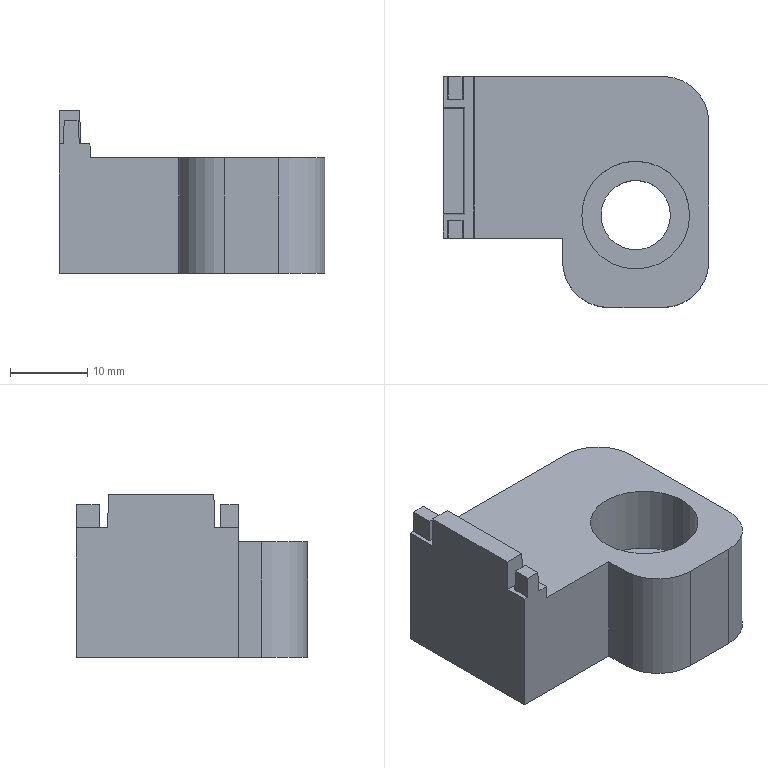Part | Creo | 1 solid | 188 faces | box 34.5 x 30 x 21.126 mm | volume 11662 mm3 | other 123 | plane 57 | cylinder 8 | commonest cylinder face diameters 12 x3 9 x2 14 x2 30.388 x1